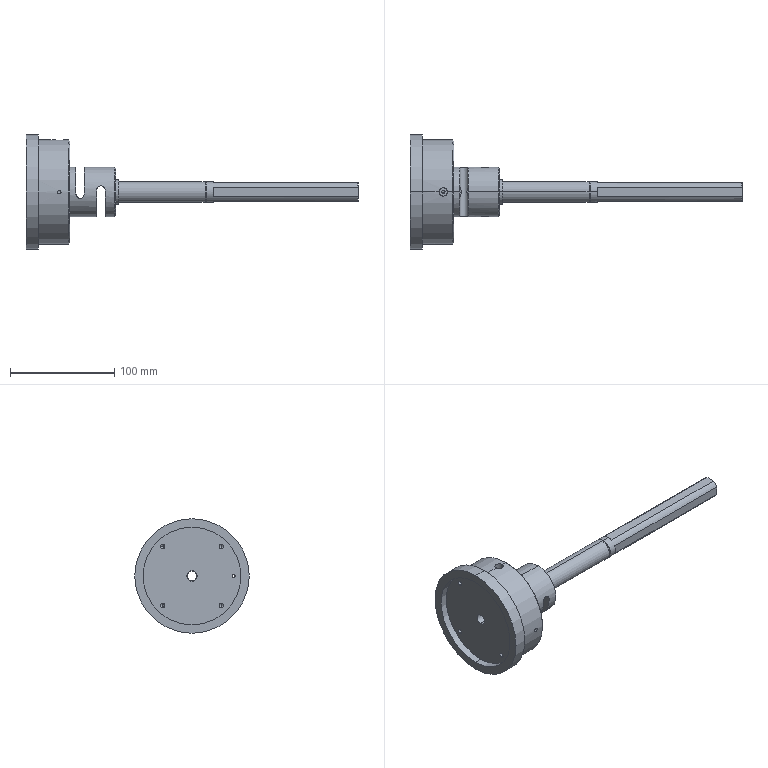Part | STEP file | longitudinal seal wheel 2_SUS304 | 2 solids | 92 faces | box 319 x 110 x 110 mm | volume 411292 mm3 | cylinder 50 | plane 26 | cone 16 | commonest cylinder face diameters 3.3 x8 4.2 x8 10 x6 8 x5 20 x4 3 x3